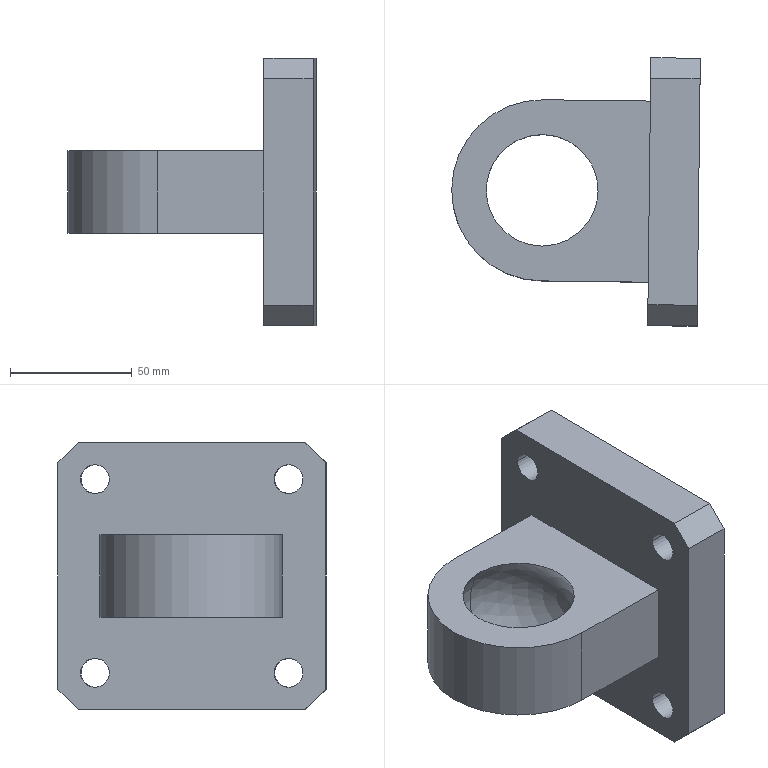Part | STEP file | Electric cylinder rear end | 1 solid | 25 faces | box 102.201 x 110.238 x 110 mm | volume 342239 mm3 | plane 14 | cylinder 9 | sphere 2 | commonest cylinder face diameters 11.846 x8 74.462 x1
STEP:
#1=CARTESIAN_POINT('',(-3113.306,-84.238,4213.637));
#2=VERTEX_POINT('',#1);
#3=CARTESIAN_POINT('',(-3113.862,-130.094,4213.637));
#4=VERTEX_POINT('',#3);
#5=CARTESIAN_POINT('',(-3113.584,-107.166,4213.637));
#6=DIRECTION('',(0.,0.,1.));
#7=DIRECTION('',(-1.,0.,0.));
#8=AXIS2_PLACEMENT_3D('',#5,#6,#7);
#9=CIRCLE('',#8,22.93);
#10=EDGE_CURVE('',#2,#4,#9,.T.);
#11=ORIENTED_EDGE('',*,*,#10,.T.);
#12=CARTESIAN_POINT('',(-3113.862,-130.094,4179.79));
#13=VERTEX_POINT('',#12);
#14=CARTESIAN_POINT('',(-3113.584,-107.166,4196.714));
#15=DIRECTION('',(0.9999,-0.01213,0.));
#16=DIRECTION('',(0.01213,0.9999,0.));
#17=AXIS2_PLACEMENT_3D('',#14,#15,#16);
#18=CIRCLE('',#17,28.499);
#19=EDGE_CURVE('',#4,#13,#18,.T.);
#20=ORIENTED_EDGE('',*,*,#19,.T.);
#21=CARTESIAN_POINT('',(-3113.306,-84.238,4179.79));
#22=VERTEX_POINT('',#21);
#23=CARTESIAN_POINT('',(-3113.584,-107.166,4179.79));
#24=DIRECTION('',(0.,0.,1.));
#25=DIRECTION('',(-1.,0.,0.));
#26=AXIS2_PLACEMENT_3D('',#23,#24,#25);
#27=CIRCLE('',#26,22.93);
#28=EDGE_CURVE('',#22,#13,#27,.T.);
#29=ORIENTED_EDGE('',*,*,#28,.F.);
#30=CARTESIAN_POINT('',(-3113.584,-107.166,4196.714));
#31=DIRECTION('',(-0.9999,0.01213,0.));
#32=DIRECTION('',(-0.01213,-0.9999,0.));
#33=AXIS2_PLACEMENT_3D('',#30,#31,#32);
#34=CIRCLE('',#33,28.499);
#35=EDGE_CURVE('',#2,#22,#34,.T.);
#36=ORIENTED_EDGE('',*,*,#35,.F.);
#37=EDGE_LOOP('',(#11,#20,#29,#36));
#38=FACE_OUTER_BOUND('',#37,.T.);
#39=CARTESIAN_POINT('',(-3113.584,-107.166,4196.714));
#40=DIRECTION('',(0.9999,-0.01213,0.));
#41=DIRECTION('',(0.01213,0.9999,0.));
#42=AXIS2_PLACEMENT_3D('',#39,#40,#41);
#43=SPHERICAL_SURFACE('',#42,28.499);
#44=ADVANCED_FACE('',(#38),#43,.F.);
#45=CARTESIAN_POINT('',(-3070.141,-153.389,4156.944));
#46=VERTEX_POINT('',#45);
#47=CARTESIAN_POINT('',(-3069.997,-141.543,4156.944));
#48=VERTEX_POINT('',#47);
#49=CARTESIAN_POINT('',(-3070.069,-147.466,4156.944));
#50=DIRECTION('',(0.9999,-0.01213,0.));
#51=DIRECTION('',(0.01213,0.9999,0.));
#52=AXIS2_PLACEMENT_3D('',#49,#50,#51);
#53=CIRCLE('',#52,5.923);
#54=EDGE_CURVE('',#46,#48,#53,.T.);
#55=ORIENTED_EDGE('',*,*,#54,.F.);
#56=CARTESIAN_POINT('',(-3049.835,-153.635,4156.944));
#57=VERTEX_POINT('',#56);
#58=CARTESIAN_POINT('',(-3049.835,-153.635,4156.944));
#59=DIRECTION('',(0.9999,-0.01213,0.));
#60=VECTOR('',#59,1000.);
#61=LINE('',#58,#60);
#62=EDGE_CURVE('',#46,#57,#61,.T.);
#63=ORIENTED_EDGE('',*,*,#62,.T.);
#64=CARTESIAN_POINT('',(-3049.691,-141.79,4156.944));
#65=VERTEX_POINT('',#64);
#66=CARTESIAN_POINT('',(-3049.763,-147.712,4156.944));
#67=DIRECTION('',(0.9999,-0.01213,0.));
#68=DIRECTION('',(0.01213,0.9999,0.));
#69=AXIS2_PLACEMENT_3D('',#66,#67,#68);
#70=CIRCLE('',#69,5.923);
#71=EDGE_CURVE('',#57,#65,#70,.T.);
#72=ORIENTED_EDGE('',*,*,#71,.T.);
#73=CARTESIAN_POINT('',(-3049.691,-141.79,4156.944));
#74=DIRECTION('',(0.9999,-0.01213,0.));
#75=VECTOR('',#74,1000.);
#76=LINE('',#73,#75);
#77=EDGE_CURVE('',#48,#65,#76,.T.);
#78=ORIENTED_EDGE('',*,*,#77,.F.);
#79=EDGE_LOOP('',(#55,#63,#72,#78));
#80=FACE_OUTER_BOUND('',#79,.T.);
#81=CARTESIAN_POINT('',(-3049.763,-147.712,4156.944));
#82=DIRECTION('',(0.9999,-0.01213,0.));
#83=DIRECTION('',(0.01213,0.9999,0.));
#84=AXIS2_PLACEMENT_3D('',#81,#82,#83);
#85=CYLINDRICAL_SURFACE('',#84,5.923);
#86=ADVANCED_FACE('',(#80),#85,.F.);
#87=CARTESIAN_POINT('',(-3069.177,-73.856,4156.944));
#88=VERTEX_POINT('',#87);
#89=CARTESIAN_POINT('',(-3069.033,-62.011,4156.944));
#90=VERTEX_POINT('',#89);
#91=CARTESIAN_POINT('',(-3069.105,-67.933,4156.944));
#92=DIRECTION('',(0.9999,-0.01213,0.));
#93=DIRECTION('',(0.01213,0.9999,0.));
#94=AXIS2_PLACEMENT_3D('',#91,#92,#93);
#95=CIRCLE('',#94,5.923);
#96=EDGE_CURVE('',#88,#90,#95,.T.);
#97=ORIENTED_EDGE('',*,*,#96,.F.);
#98=CARTESIAN_POINT('',(-3048.87,-74.102,4156.944));
#99=VERTEX_POINT('',#98);
#100=CARTESIAN_POINT('',(-3048.87,-74.102,4156.944));
#101=DIRECTION('',(0.9999,-0.01213,0.));
#102=VECTOR('',#101,1000.);
#103=LINE('',#100,#102);
#104=EDGE_CURVE('',#88,#99,#103,.T.);
#105=ORIENTED_EDGE('',*,*,#104,.T.);
#106=CARTESIAN_POINT('',(-3048.727,-62.257,4156.944));
#107=VERTEX_POINT('',#106);
#108=CARTESIAN_POINT('',(-3048.799,-68.18,4156.944));
#109=DIRECTION('',(0.9999,-0.01213,0.));
#110=DIRECTION('',(0.01213,0.9999,0.));
#111=AXIS2_PLACEMENT_3D('',#108,#109,#110);
#112=CIRCLE('',#111,5.923);
#113=EDGE_CURVE('',#99,#107,#112,.T.);
#114=ORIENTED_EDGE('',*,*,#113,.T.);
#115=CARTESIAN_POINT('',(-3048.727,-62.257,4156.944));
#116=DIRECTION('',(0.9999,-0.01213,0.));
#117=VECTOR('',#116,1000.);
#118=LINE('',#115,#117);
#119=EDGE_CURVE('',#90,#107,#118,.T.);
#120=ORIENTED_EDGE('',*,*,#119,.F.);
#121=EDGE_LOOP('',(#97,#105,#114,#120));
#122=FACE_OUTER_BOUND('',#121,.T.);
#123=CARTESIAN_POINT('',(-3048.799,-68.18,4156.944));
#124=DIRECTION('',(0.9999,-0.01213,0.));
#125=DIRECTION('',(0.01213,0.9999,0.));
#126=AXIS2_PLACEMENT_3D('',#123,#124,#125);
#127=CYLINDRICAL_SURFACE('',#126,5.923);
#128=ADVANCED_FACE('',(#122),#127,.F.);
#129=CARTESIAN_POINT('',(-3069.177,-73.856,4236.483));
#130=VERTEX_POINT('',#129);
#131=CARTESIAN_POINT('',(-3069.033,-62.011,4236.483));
#132=VERTEX_POINT('',#131);
#133=CARTESIAN_POINT('',(-3069.105,-67.933,4236.483));
#134=DIRECTION('',(0.9999,-0.01213,0.));
#135=DIRECTION('',(0.01213,0.9999,0.));
#136=AXIS2_PLACEMENT_3D('',#133,#134,#135);
#137=CIRCLE('',#136,5.923);
#138=EDGE_CURVE('',#130,#132,#137,.T.);
#139=ORIENTED_EDGE('',*,*,#138,.F.);
#140=CARTESIAN_POINT('',(-3048.87,-74.102,4236.483));
#141=VERTEX_POINT('',#140);
#142=CARTESIAN_POINT('',(-3048.87,-74.102,4236.483));
#143=DIRECTION('',(0.9999,-0.01213,0.));
#144=VECTOR('',#143,1000.);
#145=LINE('',#142,#144);
#146=EDGE_CURVE('',#130,#141,#145,.T.);
#147=ORIENTED_EDGE('',*,*,#146,.T.);
#148=CARTESIAN_POINT('',(-3048.727,-62.257,4236.483));
#149=VERTEX_POINT('',#148);
#150=CARTESIAN_POINT('',(-3048.799,-68.18,4236.483));
#151=DIRECTION('',(0.9999,-0.01213,0.));
#152=DIRECTION('',(0.01213,0.9999,0.));
#153=AXIS2_PLACEMENT_3D('',#150,#151,#152);
#154=CIRCLE('',#153,5.923);
#155=EDGE_CURVE('',#141,#149,#154,.T.);
#156=ORIENTED_EDGE('',*,*,#155,.T.);
#157=CARTESIAN_POINT('',(-3048.727,-62.257,4236.483));
#158=DIRECTION('',(0.9999,-0.01213,0.));
#159=VECTOR('',#158,1000.);
#160=LINE('',#157,#159);
#161=EDGE_CURVE('',#132,#149,#160,.T.);
#162=ORIENTED_EDGE('',*,*,#161,.F.);
#163=EDGE_LOOP('',(#139,#147,#156,#162));
#164=FACE_OUTER_BOUND('',#163,.T.);
#165=CARTESIAN_POINT('',(-3048.799,-68.18,4236.483));
#166=DIRECTION('',(0.9999,-0.01213,0.));
#167=DIRECTION('',(0.01213,0.9999,0.));
#168=AXIS2_PLACEMENT_3D('',#165,#166,#167);
#169=CYLINDRICAL_SURFACE('',#168,5.923);
#170=ADVANCED_FACE('',(#164),#169,.F.);
#171=CARTESIAN_POINT('',(-3070.141,-153.389,4236.483));
#172=VERTEX_POINT('',#171);
#173=CARTESIAN_POINT('',(-3069.997,-141.543,4236.483));
#174=VERTEX_POINT('',#173);
#175=CARTESIAN_POINT('',(-3070.069,-147.466,4236.483));
#176=DIRECTION('',(0.9999,-0.01213,0.));
#177=DIRECTION('',(0.01213,0.9999,0.));
#178=AXIS2_PLACEMENT_3D('',#175,#176,#177);
#179=CIRCLE('',#178,5.923);
#180=EDGE_CURVE('',#172,#174,#179,.T.);
#181=ORIENTED_EDGE('',*,*,#180,.F.);
#182=CARTESIAN_POINT('',(-3049.835,-153.635,4236.483));
#183=VERTEX_POINT('',#182);
#184=CARTESIAN_POINT('',(-3049.835,-153.635,4236.483));
#185=DIRECTION('',(0.9999,-0.01213,0.));
#186=VECTOR('',#185,1000.);
#187=LINE('',#184,#186);
#188=EDGE_CURVE('',#172,#183,#187,.T.);
#189=ORIENTED_EDGE('',*,*,#188,.T.);
#190=CARTESIAN_POINT('',(-3049.691,-141.79,4236.483));
#191=VERTEX_POINT('',#190);
#192=CARTESIAN_POINT('',(-3049.763,-147.712,4236.483));
#193=DIRECTION('',(0.9999,-0.01213,0.));
#194=DIRECTION('',(0.01213,0.9999,0.));
#195=AXIS2_PLACEMENT_3D('',#192,#193,#194);
#196=CIRCLE('',#195,5.923);
#197=EDGE_CURVE('',#183,#191,#196,.T.);
#198=ORIENTED_EDGE('',*,*,#197,.T.);
#199=CARTESIAN_POINT('',(-3049.691,-141.79,4236.483));
#200=DIRECTION('',(0.9999,-0.01213,0.));
#201=VECTOR('',#200,1000.);
#202=LINE('',#199,#201);
#203=EDGE_CURVE('',#174,#191,#202,.T.);
#204=ORIENTED_EDGE('',*,*,#203,.F.);
#205=EDGE_LOOP('',(#181,#189,#198,#204));
#206=FACE_OUTER_BOUND('',#205,.T.);
#207=CARTESIAN_POINT('',(-3049.763,-147.712,4236.483));
#208=DIRECTION('',(0.9999,-0.01213,0.));
#209=DIRECTION('',(0.01213,0.9999,0.));
#210=AXIS2_PLACEMENT_3D('',#207,#208,#209);
#211=CYLINDRICAL_SURFACE('',#210,5.923);
#212=ADVANCED_FACE('',(#206),#211,.F.);
#213=CARTESIAN_POINT('',(-3113.132,-69.938,4179.79));
#214=VERTEX_POINT('',#213);
#215=CARTESIAN_POINT('',(-3113.132,-69.938,4213.637));
#216=VERTEX_POINT('',#215);
#217=CARTESIAN_POINT('',(-3113.132,-69.938,4206.867));
#218=DIRECTION('',(0.,0.,1.));
#219=VECTOR('',#218,1000.);
#220=LINE('',#217,#219);
#221=EDGE_CURVE('',#214,#216,#220,.T.);
#222=ORIENTED_EDGE('',*,*,#221,.F.);
#223=CARTESIAN_POINT('',(-3114.035,-144.394,4179.79));
#224=VERTEX_POINT('',#223);
#225=CARTESIAN_POINT('',(-3113.584,-107.166,4179.79));
#226=DIRECTION('',(0.,0.,1.));
#227=DIRECTION('',(-1.,0.,0.));
#228=AXIS2_PLACEMENT_3D('',#225,#226,#227);
#229=CIRCLE('',#228,37.231);
#230=EDGE_CURVE('',#214,#224,#229,.T.);
#231=ORIENTED_EDGE('',*,*,#230,.T.);
#232=CARTESIAN_POINT('',(-3114.035,-144.394,4213.637));
#233=VERTEX_POINT('',#232);
#234=CARTESIAN_POINT('',(-3114.035,-144.394,4206.867));
#235=DIRECTION('',(0.,0.,1.));
#236=VECTOR('',#235,1000.);
#237=LINE('',#234,#236);
#238=EDGE_CURVE('',#224,#233,#237,.T.);
#239=ORIENTED_EDGE('',*,*,#238,.T.);
#240=CARTESIAN_POINT('',(-3113.584,-107.166,4213.637));
#241=DIRECTION('',(0.,0.,1.));
#242=DIRECTION('',(-1.,0.,0.));
#243=AXIS2_PLACEMENT_3D('',#240,#241,#242);
#244=CIRCLE('',#243,37.231);
#245=EDGE_CURVE('',#216,#233,#244,.T.);
#246=ORIENTED_EDGE('',*,*,#245,.F.);
#247=EDGE_LOOP('',(#222,#231,#239,#246));
#248=FACE_OUTER_BOUND('',#247,.T.);
#249=CARTESIAN_POINT('',(-3113.584,-107.166,4206.867));
#250=DIRECTION('',(0.,0.,1.));
#251=DIRECTION('',(1.,0.,0.));
#252=AXIS2_PLACEMENT_3D('',#249,#250,#251);
#253=CYLINDRICAL_SURFACE('',#252,37.231);
#254=ADVANCED_FACE('',(#248),#253,.T.);
#255=CARTESIAN_POINT('',(-3069.136,-70.472,4179.79));
#256=VERTEX_POINT('',#255);
#257=CARTESIAN_POINT('',(-3069.136,-70.472,4213.637));
#258=VERTEX_POINT('',#257);
#259=CARTESIAN_POINT('',(-3069.136,-70.472,4206.867));
#260=DIRECTION('',(0.,0.,1.));
#261=VECTOR('',#260,1000.);
#262=LINE('',#259,#261);
#263=EDGE_CURVE('',#256,#258,#262,.T.);
#264=ORIENTED_EDGE('',*,*,#263,.F.);
#265=CARTESIAN_POINT('',(-3204.51,-68.83,4179.79));
#266=DIRECTION('',(0.9999,-0.01213,0.));
#267=VECTOR('',#266,1000.);
#268=LINE('',#265,#267);
#269=EDGE_CURVE('',#214,#256,#268,.T.);
#270=ORIENTED_EDGE('',*,*,#269,.F.);
#271=ORIENTED_EDGE('',*,*,#221,.T.);
#272=CARTESIAN_POINT('',(-3204.51,-68.83,4213.637));
#273=DIRECTION('',(0.9999,-0.01213,0.));
#274=VECTOR('',#273,1000.);
#275=LINE('',#272,#274);
#276=EDGE_CURVE('',#216,#258,#275,.T.);
#277=ORIENTED_EDGE('',*,*,#276,.T.);
#278=EDGE_LOOP('',(#264,#270,#271,#277));
#279=FACE_OUTER_BOUND('',#278,.T.);
#280=CARTESIAN_POINT('',(-3069.136,-70.472,4206.867));
#281=DIRECTION('',(0.01213,0.9999,0.));
#282=DIRECTION('',(-0.9999,0.01213,0.));
#283=AXIS2_PLACEMENT_3D('',#280,#281,#282);
#284=PLANE('',#283);
#285=ADVANCED_FACE('',(#279),#284,.T.);
#286=ORIENTED_EDGE('',*,*,#238,.F.);
#287=CARTESIAN_POINT('',(-3070.038,-144.928,4179.79));
#288=VERTEX_POINT('',#287);
#289=CARTESIAN_POINT('',(-3205.413,-143.286,4179.79));
#290=DIRECTION('',(0.9999,-0.01213,0.));
#291=VECTOR('',#290,1000.);
#292=LINE('',#289,#291);
#293=EDGE_CURVE('',#224,#288,#292,.T.);
#294=ORIENTED_EDGE('',*,*,#293,.T.);
#295=CARTESIAN_POINT('',(-3070.038,-144.928,4213.637));
#296=VERTEX_POINT('',#295);
#297=CARTESIAN_POINT('',(-3070.038,-144.928,4206.867));
#298=DIRECTION('',(0.,0.,1.));
#299=VECTOR('',#298,1000.);
#300=LINE('',#297,#299);
#301=EDGE_CURVE('',#288,#296,#300,.T.);
#302=ORIENTED_EDGE('',*,*,#301,.T.);
#303=CARTESIAN_POINT('',(-3205.413,-143.286,4213.637));
#304=DIRECTION('',(0.9999,-0.01213,0.));
#305=VECTOR('',#304,1000.);
#306=LINE('',#303,#305);
#307=EDGE_CURVE('',#233,#296,#306,.T.);
#308=ORIENTED_EDGE('',*,*,#307,.F.);
#309=EDGE_LOOP('',(#286,#294,#302,#308));
#310=FACE_OUTER_BOUND('',#309,.T.);
#311=CARTESIAN_POINT('',(-3114.035,-144.394,4206.867));
#312=DIRECTION('',(-0.01213,-0.9999,0.));
#313=DIRECTION('',(0.9999,-0.01213,0.));
#314=AXIS2_PLACEMENT_3D('',#311,#312,#313);
#315=PLANE('',#314);
#316=ADVANCED_FACE('',(#310),#315,.T.);
#317=CARTESIAN_POINT('',(-3066.613,137.519,4179.79));
#318=DIRECTION('',(0.01213,0.9999,0.));
#319=VECTOR('',#318,1000.);
#320=LINE('',#317,#319);
#321=EDGE_CURVE('',#288,#256,#320,.T.);
#322=ORIENTED_EDGE('',*,*,#321,.T.);
#323=ORIENTED_EDGE('',*,*,#263,.T.);
#324=CARTESIAN_POINT('',(-3066.613,137.519,4213.637));
#325=DIRECTION('',(0.01213,0.9999,0.));
#326=VECTOR('',#325,1000.);
#327=LINE('',#324,#326);
#328=EDGE_CURVE('',#296,#258,#327,.T.);
#329=ORIENTED_EDGE('',*,*,#328,.F.);
#330=ORIENTED_EDGE('',*,*,#301,.F.);
#331=EDGE_LOOP('',(#322,#323,#329,#330));
#332=FACE_BOUND('',#331,.T.);
#333=CARTESIAN_POINT('',(-3070.254,-162.696,4243.252));
#334=VERTEX_POINT('',#333);
#335=CARTESIAN_POINT('',(-3070.254,-162.696,4150.175));
#336=VERTEX_POINT('',#335);
#337=CARTESIAN_POINT('',(-3070.254,-162.696,4251.714));
#338=DIRECTION('',(0.,0.,-1.));
#339=VECTOR('',#338,1000.);
#340=LINE('',#337,#339);
#341=EDGE_CURVE('',#334,#336,#340,.T.);
#342=ORIENTED_EDGE('',*,*,#341,.F.);
#343=CARTESIAN_POINT('',(-3070.151,-154.235,4251.714));
#344=VERTEX_POINT('',#343);
#345=CARTESIAN_POINT('',(-3070.151,-154.235,4251.714));
#346=DIRECTION('',(0.008574,0.7071,0.7071));
#347=VECTOR('',#346,1000.);
#348=LINE('',#345,#347);
#349=EDGE_CURVE('',#334,#344,#348,.T.);
#350=ORIENTED_EDGE('',*,*,#349,.T.);
#351=CARTESIAN_POINT('',(-3069.023,-61.165,4251.714));
#352=VERTEX_POINT('',#351);
#353=CARTESIAN_POINT('',(-3068.92,-52.704,4251.714));
#354=DIRECTION('',(-0.01213,-0.9999,0.));
#355=VECTOR('',#354,1000.);
#356=LINE('',#353,#355);
#357=EDGE_CURVE('',#352,#344,#356,.T.);
#358=ORIENTED_EDGE('',*,*,#357,.F.);
#359=CARTESIAN_POINT('',(-3068.92,-52.704,4243.252));
#360=VERTEX_POINT('',#359);
#361=CARTESIAN_POINT('',(-3068.92,-52.704,4243.252));
#362=DIRECTION('',(0.008574,0.7071,-0.7071));
#363=VECTOR('',#362,1000.);
#364=LINE('',#361,#363);
#365=EDGE_CURVE('',#352,#360,#364,.T.);
#366=ORIENTED_EDGE('',*,*,#365,.T.);
#367=CARTESIAN_POINT('',(-3068.92,-52.704,4150.175));
#368=VERTEX_POINT('',#367);
#369=CARTESIAN_POINT('',(-3068.92,-52.704,4141.714));
#370=DIRECTION('',(0.,0.,1.));
#371=VECTOR('',#370,1000.);
#372=LINE('',#369,#371);
#373=EDGE_CURVE('',#368,#360,#372,.T.);
#374=ORIENTED_EDGE('',*,*,#373,.F.);
#375=CARTESIAN_POINT('',(-3069.023,-61.165,4141.714));
#376=VERTEX_POINT('',#375);
#377=CARTESIAN_POINT('',(-3069.023,-61.165,4141.714));
#378=DIRECTION('',(-0.008574,-0.7071,-0.7071));
#379=VECTOR('',#378,1000.);
#380=LINE('',#377,#379);
#381=EDGE_CURVE('',#368,#376,#380,.T.);
#382=ORIENTED_EDGE('',*,*,#381,.T.);
#383=CARTESIAN_POINT('',(-3070.151,-154.235,4141.714));
#384=VERTEX_POINT('',#383);
#385=CARTESIAN_POINT('',(-3070.254,-162.696,4141.714));
#386=DIRECTION('',(0.01213,0.9999,0.));
#387=VECTOR('',#386,1000.);
#388=LINE('',#385,#387);
#389=EDGE_CURVE('',#384,#376,#388,.T.);
#390=ORIENTED_EDGE('',*,*,#389,.F.);
#391=CARTESIAN_POINT('',(-3070.254,-162.696,4150.175));
#392=DIRECTION('',(-0.008574,-0.7071,0.7071));
#393=VECTOR('',#392,1000.);
#394=LINE('',#391,#393);
#395=EDGE_CURVE('',#384,#336,#394,.T.);
#396=ORIENTED_EDGE('',*,*,#395,.T.);
#397=EDGE_LOOP('',(#342,#350,#358,#366,#374,#382,#390,#396));
#398=FACE_OUTER_BOUND('',#397,.T.);
#399=CARTESIAN_POINT('',(-3070.069,-147.466,4236.483));
#400=DIRECTION('',(0.9999,-0.01213,0.));
#401=DIRECTION('',(0.01213,0.9999,0.));
#402=AXIS2_PLACEMENT_3D('',#399,#400,#401);
#403=CIRCLE('',#402,5.923);
#404=EDGE_CURVE('',#174,#172,#403,.T.);
#405=ORIENTED_EDGE('',*,*,#404,.T.);
#406=ORIENTED_EDGE('',*,*,#180,.T.);
#407=EDGE_LOOP('',(#405,#406));
#408=FACE_BOUND('',#407,.T.);
#409=CARTESIAN_POINT('',(-3069.105,-67.933,4236.483));
#410=DIRECTION('',(0.9999,-0.01213,0.));
#411=DIRECTION('',(0.01213,0.9999,0.));
#412=AXIS2_PLACEMENT_3D('',#409,#410,#411);
#413=CIRCLE('',#412,5.923);
#414=EDGE_CURVE('',#132,#130,#413,.T.);
#415=ORIENTED_EDGE('',*,*,#414,.T.);
#416=ORIENTED_EDGE('',*,*,#138,.T.);
#417=EDGE_LOOP('',(#415,#416));
#418=FACE_BOUND('',#417,.T.);
#419=CARTESIAN_POINT('',(-3069.105,-67.933,4156.944));
#420=DIRECTION('',(0.9999,-0.01213,0.));
#421=DIRECTION('',(0.01213,0.9999,0.));
#422=AXIS2_PLACEMENT_3D('',#419,#420,#421);
#423=CIRCLE('',#422,5.923);
#424=EDGE_CURVE('',#90,#88,#423,.T.);
#425=ORIENTED_EDGE('',*,*,#424,.T.);
#426=ORIENTED_EDGE('',*,*,#96,.T.);
#427=EDGE_LOOP('',(#425,#426));
#428=FACE_BOUND('',#427,.T.);
#429=CARTESIAN_POINT('',(-3070.069,-147.466,4156.944));
#430=DIRECTION('',(0.9999,-0.01213,0.));
#431=DIRECTION('',(0.01213,0.9999,0.));
#432=AXIS2_PLACEMENT_3D('',#429,#430,#431);
#433=CIRCLE('',#432,5.923);
#434=EDGE_CURVE('',#48,#46,#433,.T.);
#435=ORIENTED_EDGE('',*,*,#434,.T.);
#436=ORIENTED_EDGE('',*,*,#54,.T.);
#437=EDGE_LOOP('',(#435,#436));
#438=FACE_BOUND('',#437,.T.);
#439=CARTESIAN_POINT('',(-3066.613,137.519,-2905.417));
#440=DIRECTION('',(0.9999,-0.01213,0.));
#441=DIRECTION('',(0.01213,0.9999,0.));
#442=AXIS2_PLACEMENT_3D('',#439,#440,#441);
#443=PLANE('',#442);
#444=ADVANCED_FACE('',(#332,#398,#408,#418,#428,#438),#443,.F.);
#445=ORIENTED_EDGE('',*,*,#373,.T.);
#446=CARTESIAN_POINT('',(-3048.614,-52.95,4243.252));
#447=VERTEX_POINT('',#446);
#448=CARTESIAN_POINT('',(-3068.92,-52.704,4243.252));
#449=DIRECTION('',(0.9999,-0.01213,0.));
#450=VECTOR('',#449,1000.);
#451=LINE('',#448,#450);
#452=EDGE_CURVE('',#360,#447,#451,.T.);
#453=ORIENTED_EDGE('',*,*,#452,.T.);
#454=CARTESIAN_POINT('',(-3048.614,-52.95,4150.175));
#455=VERTEX_POINT('',#454);
#456=CARTESIAN_POINT('',(-3048.614,-52.95,4141.714));
#457=DIRECTION('',(0.,0.,1.));
#458=VECTOR('',#457,1000.);
#459=LINE('',#456,#458);
#460=EDGE_CURVE('',#455,#447,#459,.T.);
#461=ORIENTED_EDGE('',*,*,#460,.F.);
#462=CARTESIAN_POINT('',(-3068.92,-52.704,4150.175));
#463=DIRECTION('',(-0.9999,0.01213,0.));
#464=VECTOR('',#463,1000.);
#465=LINE('',#462,#464);
#466=EDGE_CURVE('',#455,#368,#465,.T.);
#467=ORIENTED_EDGE('',*,*,#466,.T.);
#468=EDGE_LOOP('',(#445,#453,#461,#467));
#469=FACE_OUTER_BOUND('',#468,.T.);
#470=CARTESIAN_POINT('',(-3068.92,-52.704,4141.714));
#471=DIRECTION('',(0.01213,0.9999,0.));
#472=DIRECTION('',(-0.9999,0.01213,0.));
#473=AXIS2_PLACEMENT_3D('',#470,#471,#472);
#474=PLANE('',#473);
#475=ADVANCED_FACE('',(#469),#474,.T.);
#476=ORIENTED_EDGE('',*,*,#389,.T.);
#477=CARTESIAN_POINT('',(-3048.717,-61.411,4141.714));
#478=VERTEX_POINT('',#477);
#479=CARTESIAN_POINT('',(-3069.023,-61.165,4141.714));
#480=DIRECTION('',(0.9999,-0.01213,0.));
#481=VECTOR('',#480,1000.);
#482=LINE('',#479,#481);
#483=EDGE_CURVE('',#376,#478,#482,.T.);
#484=ORIENTED_EDGE('',*,*,#483,.T.);
#485=CARTESIAN_POINT('',(-3049.845,-154.481,4141.714));
#486=VERTEX_POINT('',#485);
#487=CARTESIAN_POINT('',(-3049.948,-162.942,4141.714));
#488=DIRECTION('',(0.01213,0.9999,0.));
#489=VECTOR('',#488,1000.);
#490=LINE('',#487,#489);
#491=EDGE_CURVE('',#486,#478,#490,.T.);
#492=ORIENTED_EDGE('',*,*,#491,.F.);
#493=CARTESIAN_POINT('',(-3070.151,-154.235,4141.714));
#494=DIRECTION('',(-0.9999,0.01213,0.));
#495=VECTOR('',#494,1000.);
#496=LINE('',#493,#495);
#497=EDGE_CURVE('',#486,#384,#496,.T.);
#498=ORIENTED_EDGE('',*,*,#497,.T.);
#499=EDGE_LOOP('',(#476,#484,#492,#498));
#500=FACE_OUTER_BOUND('',#499,.T.);
#501=CARTESIAN_POINT('',(-3070.254,-162.696,4141.714));
#502=DIRECTION('',(0.,0.,-1.));
#503=DIRECTION('',(-1.,0.,0.));
#504=AXIS2_PLACEMENT_3D('',#501,#502,#503);
#505=PLANE('',#504);
#506=ADVANCED_FACE('',(#500),#505,.T.);
#507=CARTESIAN_POINT('',(-3049.948,-162.942,4243.252));
#508=VERTEX_POINT('',#507);
#509=CARTESIAN_POINT('',(-3049.948,-162.942,4150.175));
#510=VERTEX_POINT('',#509);
#511=CARTESIAN_POINT('',(-3049.948,-162.942,4251.714));
#512=DIRECTION('',(0.,0.,-1.));
#513=VECTOR('',#512,1000.);
#514=LINE('',#511,#513);
#515=EDGE_CURVE('',#508,#510,#514,.T.);
#516=ORIENTED_EDGE('',*,*,#515,.F.);
#517=CARTESIAN_POINT('',(-3070.254,-162.696,4243.252));
#518=DIRECTION('',(-0.9999,0.01213,0.));
#519=VECTOR('',#518,1000.);
#520=LINE('',#517,#519);
#521=EDGE_CURVE('',#508,#334,#520,.T.);
#522=ORIENTED_EDGE('',*,*,#521,.T.);
#523=ORIENTED_EDGE('',*,*,#341,.T.);
#524=CARTESIAN_POINT('',(-3070.254,-162.696,4150.175));
#525=DIRECTION('',(0.9999,-0.01213,0.));
#526=VECTOR('',#525,1000.);
#527=LINE('',#524,#526);
#528=EDGE_CURVE('',#336,#510,#527,.T.);
#529=ORIENTED_EDGE('',*,*,#528,.T.);
#530=EDGE_LOOP('',(#516,#522,#523,#529));
#531=FACE_OUTER_BOUND('',#530,.T.);
#532=CARTESIAN_POINT('',(-3070.254,-162.696,4251.714));
#533=DIRECTION('',(-0.01213,-0.9999,0.));
#534=DIRECTION('',(0.9999,-0.01213,0.));
#535=AXIS2_PLACEMENT_3D('',#532,#533,#534);
#536=PLANE('',#535);
#537=ADVANCED_FACE('',(#531),#536,.T.);
#538=ORIENTED_EDGE('',*,*,#357,.T.);
#539=CARTESIAN_POINT('',(-3049.845,-154.481,4251.714));
#540=VERTEX_POINT('',#539);
#541=CARTESIAN_POINT('',(-3070.151,-154.235,4251.714));
#542=DIRECTION('',(0.9999,-0.01213,0.));
#543=VECTOR('',#542,1000.);
#544=LINE('',#541,#543);
#545=EDGE_CURVE('',#344,#540,#544,.T.);
#546=ORIENTED_EDGE('',*,*,#545,.T.);
#547=CARTESIAN_POINT('',(-3048.717,-61.411,4251.714));
#548=VERTEX_POINT('',#547);
#549=CARTESIAN_POINT('',(-3048.614,-52.95,4251.714));
#550=DIRECTION('',(-0.01213,-0.9999,0.));
#551=VECTOR('',#550,1000.);
#552=LINE('',#549,#551);
#553=EDGE_CURVE('',#548,#540,#552,.T.);
#554=ORIENTED_EDGE('',*,*,#553,.F.);
#555=CARTESIAN_POINT('',(-3069.023,-61.165,4251.714));
#556=DIRECTION('',(-0.9999,0.01213,0.));
#557=VECTOR('',#556,1000.);
#558=LINE('',#555,#557);
#559=EDGE_CURVE('',#548,#352,#558,.T.);
#560=ORIENTED_EDGE('',*,*,#559,.T.);
#561=EDGE_LOOP('',(#538,#546,#554,#560));
#562=FACE_OUTER_BOUND('',#561,.T.);
#563=CARTESIAN_POINT('',(-3068.92,-52.704,4251.714));
#564=DIRECTION('',(0.,0.,1.));
#565=DIRECTION('',(1.,0.,0.));
#566=AXIS2_PLACEMENT_3D('',#563,#564,#565);
#567=PLANE('',#566);
#568=ADVANCED_FACE('',(#562),#567,.T.);
#569=CARTESIAN_POINT('',(-3049.763,-147.712,4156.944));
#570=DIRECTION('',(0.9999,-0.01213,0.));
#571=DIRECTION('',(0.01213,0.9999,0.));
#572=AXIS2_PLACEMENT_3D('',#569,#570,#571);
#573=CIRCLE('',#572,5.923);
#574=EDGE_CURVE('',#65,#57,#573,.T.);
#575=ORIENTED_EDGE('',*,*,#574,.F.);
#576=ORIENTED_EDGE('',*,*,#71,.F.);
#577=EDGE_LOOP('',(#575,#576));
#578=FACE_BOUND('',#577,.T.);
#579=CARTESIAN_POINT('',(-3048.799,-68.18,4156.944));
#580=DIRECTION('',(0.9999,-0.01213,0.));
#581=DIRECTION('',(0.01213,0.9999,0.));
#582=AXIS2_PLACEMENT_3D('',#579,#580,#581);
#583=CIRCLE('',#582,5.923);
#584=EDGE_CURVE('',#107,#99,#583,.T.);
#585=ORIENTED_EDGE('',*,*,#584,.F.);
#586=ORIENTED_EDGE('',*,*,#113,.F.);
#587=EDGE_LOOP('',(#585,#586));
#588=FACE_BOUND('',#587,.T.);
#589=CARTESIAN_POINT('',(-3048.799,-68.18,4236.483));
#590=DIRECTION('',(0.9999,-0.01213,0.));
#591=DIRECTION('',(0.01213,0.9999,0.));
#592=AXIS2_PLACEMENT_3D('',#589,#590,#591);
#593=CIRCLE('',#592,5.923);
#594=EDGE_CURVE('',#149,#141,#593,.T.);
#595=ORIENTED_EDGE('',*,*,#594,.F.);
#596=ORIENTED_EDGE('',*,*,#155,.F.);
#597=EDGE_LOOP('',(#595,#596));
#598=FACE_BOUND('',#597,.T.);
#599=CARTESIAN_POINT('',(-3049.763,-147.712,4236.483));
#600=DIRECTION('',(0.9999,-0.01213,0.));
#601=DIRECTION('',(0.01213,0.9999,0.));
#602=AXIS2_PLACEMENT_3D('',#599,#600,#601);
#603=CIRCLE('',#602,5.923);
#604=EDGE_CURVE('',#191,#183,#603,.T.);
#605=ORIENTED_EDGE('',*,*,#604,.F.);
#606=ORIENTED_EDGE('',*,*,#197,.F.);
#607=EDGE_LOOP('',(#605,#606));
#608=FACE_BOUND('',#607,.T.);
#609=ORIENTED_EDGE('',*,*,#553,.T.);
#610=CARTESIAN_POINT('',(-3091.469,-3586.906,819.036));
#611=DIRECTION('',(-0.008574,-0.7071,-0.7071));
#612=VECTOR('',#611,1000.);
#613=LINE('',#610,#612);
#614=EDGE_CURVE('',#540,#508,#613,.T.);
#615=ORIENTED_EDGE('',*,*,#614,.T.);
#616=ORIENTED_EDGE('',*,*,#515,.T.);
#617=CARTESIAN_POINT('',(-3005.351,3514.702,472.261));
#618=DIRECTION('',(0.008574,0.7071,-0.7071));
#619=VECTOR('',#618,1000.);
#620=LINE('',#617,#619);
#621=EDGE_CURVE('',#510,#486,#620,.T.);
#622=ORIENTED_EDGE('',*,*,#621,.T.);
#623=ORIENTED_EDGE('',*,*,#491,.T.);
#624=CARTESIAN_POINT('',(-3090.237,-3485.375,717.497));
#625=DIRECTION('',(0.008574,0.7071,0.7071));
#626=VECTOR('',#625,1000.);
#627=LINE('',#624,#626);
#628=EDGE_CURVE('',#478,#455,#627,.T.);
#629=ORIENTED_EDGE('',*,*,#628,.T.);
#630=ORIENTED_EDGE('',*,*,#460,.T.);
#631=CARTESIAN_POINT('',(-3004.119,3616.233,573.799));
#632=DIRECTION('',(-0.008574,-0.7071,0.7071));
#633=VECTOR('',#632,1000.);
#634=LINE('',#631,#633);
#635=EDGE_CURVE('',#447,#548,#634,.T.);
#636=ORIENTED_EDGE('',*,*,#635,.T.);
#637=EDGE_LOOP('',(#609,#615,#616,#622,#623,#629,#630,#636));
#638=FACE_OUTER_BOUND('',#637,.T.);
#639=CARTESIAN_POINT('',(-3046.307,137.273,-2905.417));
#640=DIRECTION('',(0.9999,-0.01213,0.));
#641=DIRECTION('',(0.01213,0.9999,0.));
#642=AXIS2_PLACEMENT_3D('',#639,#640,#641);
#643=PLANE('',#642);
#644=ADVANCED_FACE('',(#578,#588,#598,#608,#638),#643,.T.);
#645=ORIENTED_EDGE('',*,*,#188,.F.);
#646=ORIENTED_EDGE('',*,*,#404,.F.);
#647=ORIENTED_EDGE('',*,*,#203,.T.);
#648=ORIENTED_EDGE('',*,*,#604,.T.);
#649=EDGE_LOOP('',(#645,#646,#647,#648));
#650=FACE_OUTER_BOUND('',#649,.T.);
#651=CARTESIAN_POINT('',(-3049.763,-147.712,4236.483));
#652=DIRECTION('',(0.9999,-0.01213,0.));
#653=DIRECTION('',(0.01213,0.9999,0.));
#654=AXIS2_PLACEMENT_3D('',#651,#652,#653);
#655=CYLINDRICAL_SURFACE('',#654,5.923);
#656=ADVANCED_FACE('',(#650),#655,.F.);
#657=ORIENTED_EDGE('',*,*,#146,.F.);
#658=ORIENTED_EDGE('',*,*,#414,.F.);
#659=ORIENTED_EDGE('',*,*,#161,.T.);
#660=ORIENTED_EDGE('',*,*,#594,.T.);
#661=EDGE_LOOP('',(#657,#658,#659,#660));
#662=FACE_OUTER_BOUND('',#661,.T.);
#663=CARTESIAN_POINT('',(-3048.799,-68.18,4236.483));
#664=DIRECTION('',(0.9999,-0.01213,0.));
#665=DIRECTION('',(0.01213,0.9999,0.));
#666=AXIS2_PLACEMENT_3D('',#663,#664,#665);
#667=CYLINDRICAL_SURFACE('',#666,5.923);
#668=ADVANCED_FACE('',(#662),#667,.F.);
#669=ORIENTED_EDGE('',*,*,#104,.F.);
#670=ORIENTED_EDGE('',*,*,#424,.F.);
#671=ORIENTED_EDGE('',*,*,#119,.T.);
#672=ORIENTED_EDGE('',*,*,#584,.T.);
#673=EDGE_LOOP('',(#669,#670,#671,#672));
#674=FACE_OUTER_BOUND('',#673,.T.);
#675=CARTESIAN_POINT('',(-3048.799,-68.18,4156.944));
#676=DIRECTION('',(0.9999,-0.01213,0.));
#677=DIRECTION('',(0.01213,0.9999,0.));
#678=AXIS2_PLACEMENT_3D('',#675,#676,#677);
#679=CYLINDRICAL_SURFACE('',#678,5.923);
#680=ADVANCED_FACE('',(#674),#679,.F.);
#681=ORIENTED_EDGE('',*,*,#62,.F.);
#682=ORIENTED_EDGE('',*,*,#434,.F.);
#683=ORIENTED_EDGE('',*,*,#77,.T.);
#684=ORIENTED_EDGE('',*,*,#574,.T.);
#685=EDGE_LOOP('',(#681,#682,#683,#684));
#686=FACE_OUTER_BOUND('',#685,.T.);
#687=CARTESIAN_POINT('',(-3049.763,-147.712,4156.944));
#688=DIRECTION('',(0.9999,-0.01213,0.));
#689=DIRECTION('',(0.01213,0.9999,0.));
#690=AXIS2_PLACEMENT_3D('',#687,#688,#689);
#691=CYLINDRICAL_SURFACE('',#690,5.923);
#692=ADVANCED_FACE('',(#686),#691,.F.);
#693=ORIENTED_EDGE('',*,*,#349,.F.);
#694=ORIENTED_EDGE('',*,*,#521,.F.);
#695=ORIENTED_EDGE('',*,*,#614,.F.);
#696=ORIENTED_EDGE('',*,*,#545,.F.);
#697=EDGE_LOOP('',(#693,#694,#695,#696));
#698=FACE_OUTER_BOUND('',#697,.T.);
#699=CARTESIAN_POINT('',(-3070.151,-154.235,4251.714));
#700=DIRECTION('',(0.008574,0.7071,-0.7071));
#701=DIRECTION('',(0.9999,-0.01213,0.));
#702=AXIS2_PLACEMENT_3D('',#699,#700,#701);
#703=PLANE('',#702);
#704=ADVANCED_FACE('',(#698),#703,.F.);
#705=ORIENTED_EDGE('',*,*,#365,.F.);
#706=ORIENTED_EDGE('',*,*,#559,.F.);
#707=ORIENTED_EDGE('',*,*,#635,.F.);
#708=ORIENTED_EDGE('',*,*,#452,.F.);
#709=EDGE_LOOP('',(#705,#706,#707,#708));
#710=FACE_OUTER_BOUND('',#709,.T.);
#711=CARTESIAN_POINT('',(-3068.92,-52.704,4243.252));
#712=DIRECTION('',(-0.008574,-0.7071,-0.7071));
#713=DIRECTION('',(0.9999,-0.01213,0.));
#714=AXIS2_PLACEMENT_3D('',#711,#712,#713);
#715=PLANE('',#714);
#716=ADVANCED_FACE('',(#710),#715,.F.);
#717=ORIENTED_EDGE('',*,*,#381,.F.);
#718=ORIENTED_EDGE('',*,*,#466,.F.);
#719=ORIENTED_EDGE('',*,*,#628,.F.);
#720=ORIENTED_EDGE('',*,*,#483,.F.);
#721=EDGE_LOOP('',(#717,#718,#719,#720));
#722=FACE_OUTER_BOUND('',#721,.T.);
#723=CARTESIAN_POINT('',(-3069.023,-61.165,4141.714));
#724=DIRECTION('',(-0.008574,-0.7071,0.7071));
#725=DIRECTION('',(0.9999,-0.01213,0.));
#726=AXIS2_PLACEMENT_3D('',#723,#724,#725);
#727=PLANE('',#726);
#728=ADVANCED_FACE('',(#722),#727,.F.);
#729=ORIENTED_EDGE('',*,*,#395,.F.);
#730=ORIENTED_EDGE('',*,*,#497,.F.);
#731=ORIENTED_EDGE('',*,*,#621,.F.);
#732=ORIENTED_EDGE('',*,*,#528,.F.);
#733=EDGE_LOOP('',(#729,#730,#731,#732));
#734=FACE_OUTER_BOUND('',#733,.T.);
#735=CARTESIAN_POINT('',(-3070.254,-162.696,4150.175));
#736=DIRECTION('',(0.008574,0.7071,0.7071));
#737=DIRECTION('',(0.9999,-0.01213,0.));
#738=AXIS2_PLACEMENT_3D('',#735,#736,#737);
#739=PLANE('',#738);
#740=ADVANCED_FACE('',(#734),#739,.F.);
#741=ORIENTED_EDGE('',*,*,#245,.T.);
#742=ORIENTED_EDGE('',*,*,#307,.T.);
#743=ORIENTED_EDGE('',*,*,#328,.T.);
#744=ORIENTED_EDGE('',*,*,#276,.F.);
#745=EDGE_LOOP('',(#741,#742,#743,#744));
#746=FACE_OUTER_BOUND('',#745,.T.);
#747=ORIENTED_EDGE('',*,*,#10,.F.);
#748=CARTESIAN_POINT('',(-3113.584,-107.166,4213.637));
#749=DIRECTION('',(0.,0.,1.));
#750=DIRECTION('',(-1.,0.,0.));
#751=AXIS2_PLACEMENT_3D('',#748,#749,#750);
#752=CIRCLE('',#751,22.93);
#753=EDGE_CURVE('',#4,#2,#752,.T.);
#754=ORIENTED_EDGE('',*,*,#753,.F.);
#755=EDGE_LOOP('',(#747,#754));
#756=FACE_BOUND('',#755,.T.);
#757=CARTESIAN_POINT('',(-3201.988,139.161,4213.637));
#758=DIRECTION('',(0.,0.,-1.));
#759=DIRECTION('',(-1.,0.,0.));
#760=AXIS2_PLACEMENT_3D('',#757,#758,#759);
#761=PLANE('',#760);
#762=ADVANCED_FACE('',(#746,#756),#761,.F.);
#763=ORIENTED_EDGE('',*,*,#269,.T.);
#764=ORIENTED_EDGE('',*,*,#321,.F.);
#765=ORIENTED_EDGE('',*,*,#293,.F.);
#766=ORIENTED_EDGE('',*,*,#230,.F.);
#767=EDGE_LOOP('',(#763,#764,#765,#766));
#768=FACE_OUTER_BOUND('',#767,.T.);
#769=ORIENTED_EDGE('',*,*,#28,.T.);
#770=CARTESIAN_POINT('',(-3113.584,-107.166,4179.79));
#771=DIRECTION('',(0.,0.,1.));
#772=DIRECTION('',(-1.,0.,0.));
#773=AXIS2_PLACEMENT_3D('',#770,#771,#772);
#774=CIRCLE('',#773,22.93);
#775=EDGE_CURVE('',#13,#22,#774,.T.);
#776=ORIENTED_EDGE('',*,*,#775,.T.);
#777=EDGE_LOOP('',(#769,#776));
#778=FACE_BOUND('',#777,.T.);
#779=CARTESIAN_POINT('',(-3201.988,139.161,4179.79));
#780=DIRECTION('',(0.,0.,-1.));
#781=DIRECTION('',(-1.,0.,0.));
#782=AXIS2_PLACEMENT_3D('',#779,#780,#781);
#783=PLANE('',#782);
#784=ADVANCED_FACE('',(#768,#778),#783,.T.);
#785=ORIENTED_EDGE('',*,*,#19,.F.);
#786=ORIENTED_EDGE('',*,*,#753,.T.);
#787=ORIENTED_EDGE('',*,*,#35,.T.);
#788=ORIENTED_EDGE('',*,*,#775,.F.);
#789=EDGE_LOOP('',(#785,#786,#787,#788));
#790=FACE_OUTER_BOUND('',#789,.T.);
#791=CARTESIAN_POINT('',(-3113.584,-107.166,4196.714));
#792=DIRECTION('',(0.9999,-0.01213,0.));
#793=DIRECTION('',(0.01213,0.9999,0.));
#794=AXIS2_PLACEMENT_3D('',#791,#792,#793);
#795=SPHERICAL_SURFACE('',#794,28.499);
#796=ADVANCED_FACE('',(#790),#795,.F.);
#797=CLOSED_SHELL('',(#44,#86,#128,#170,#212,#254,#285,#316,#444,#475,#506,#537,#568,#644,#656,#668,#680,#692,#704,#716,#728,#740,#762,#784,#796));
#798=MANIFOLD_SOLID_BREP('',#797);
#799=CARTESIAN_POINT('',(0.,0.,0.));
#800=DIRECTION('',(0.,0.,1.));
#801=DIRECTION('',(1.,0.,0.));
#802=AXIS2_PLACEMENT_3D('',#799,#800,#801);
#803=(LENGTH_UNIT()NAMED_UNIT(*)SI_UNIT(.MILLI.,.METRE.));
#804=UNCERTAINTY_MEASURE_WITH_UNIT(LENGTH_MEASURE(0.00001),#803,'','');
#805=(NAMED_UNIT(*)PLANE_ANGLE_UNIT()SI_UNIT($,.RADIAN.));
#806=(NAMED_UNIT(*)SI_UNIT($,.STERADIAN.)SOLID_ANGLE_UNIT());
#807=(GEOMETRIC_REPRESENTATION_CONTEXT(3)GLOBAL_UNCERTAINTY_ASSIGNED_CONTEXT((#804))GLOBAL_UNIT_ASSIGNED_CONTEXT((#803,#805,#806))REPRESENTATION_CONTEXT('',''));
#808=ADVANCED_BREP_SHAPE_REPRESENTATION('',(#798,#802),#807);